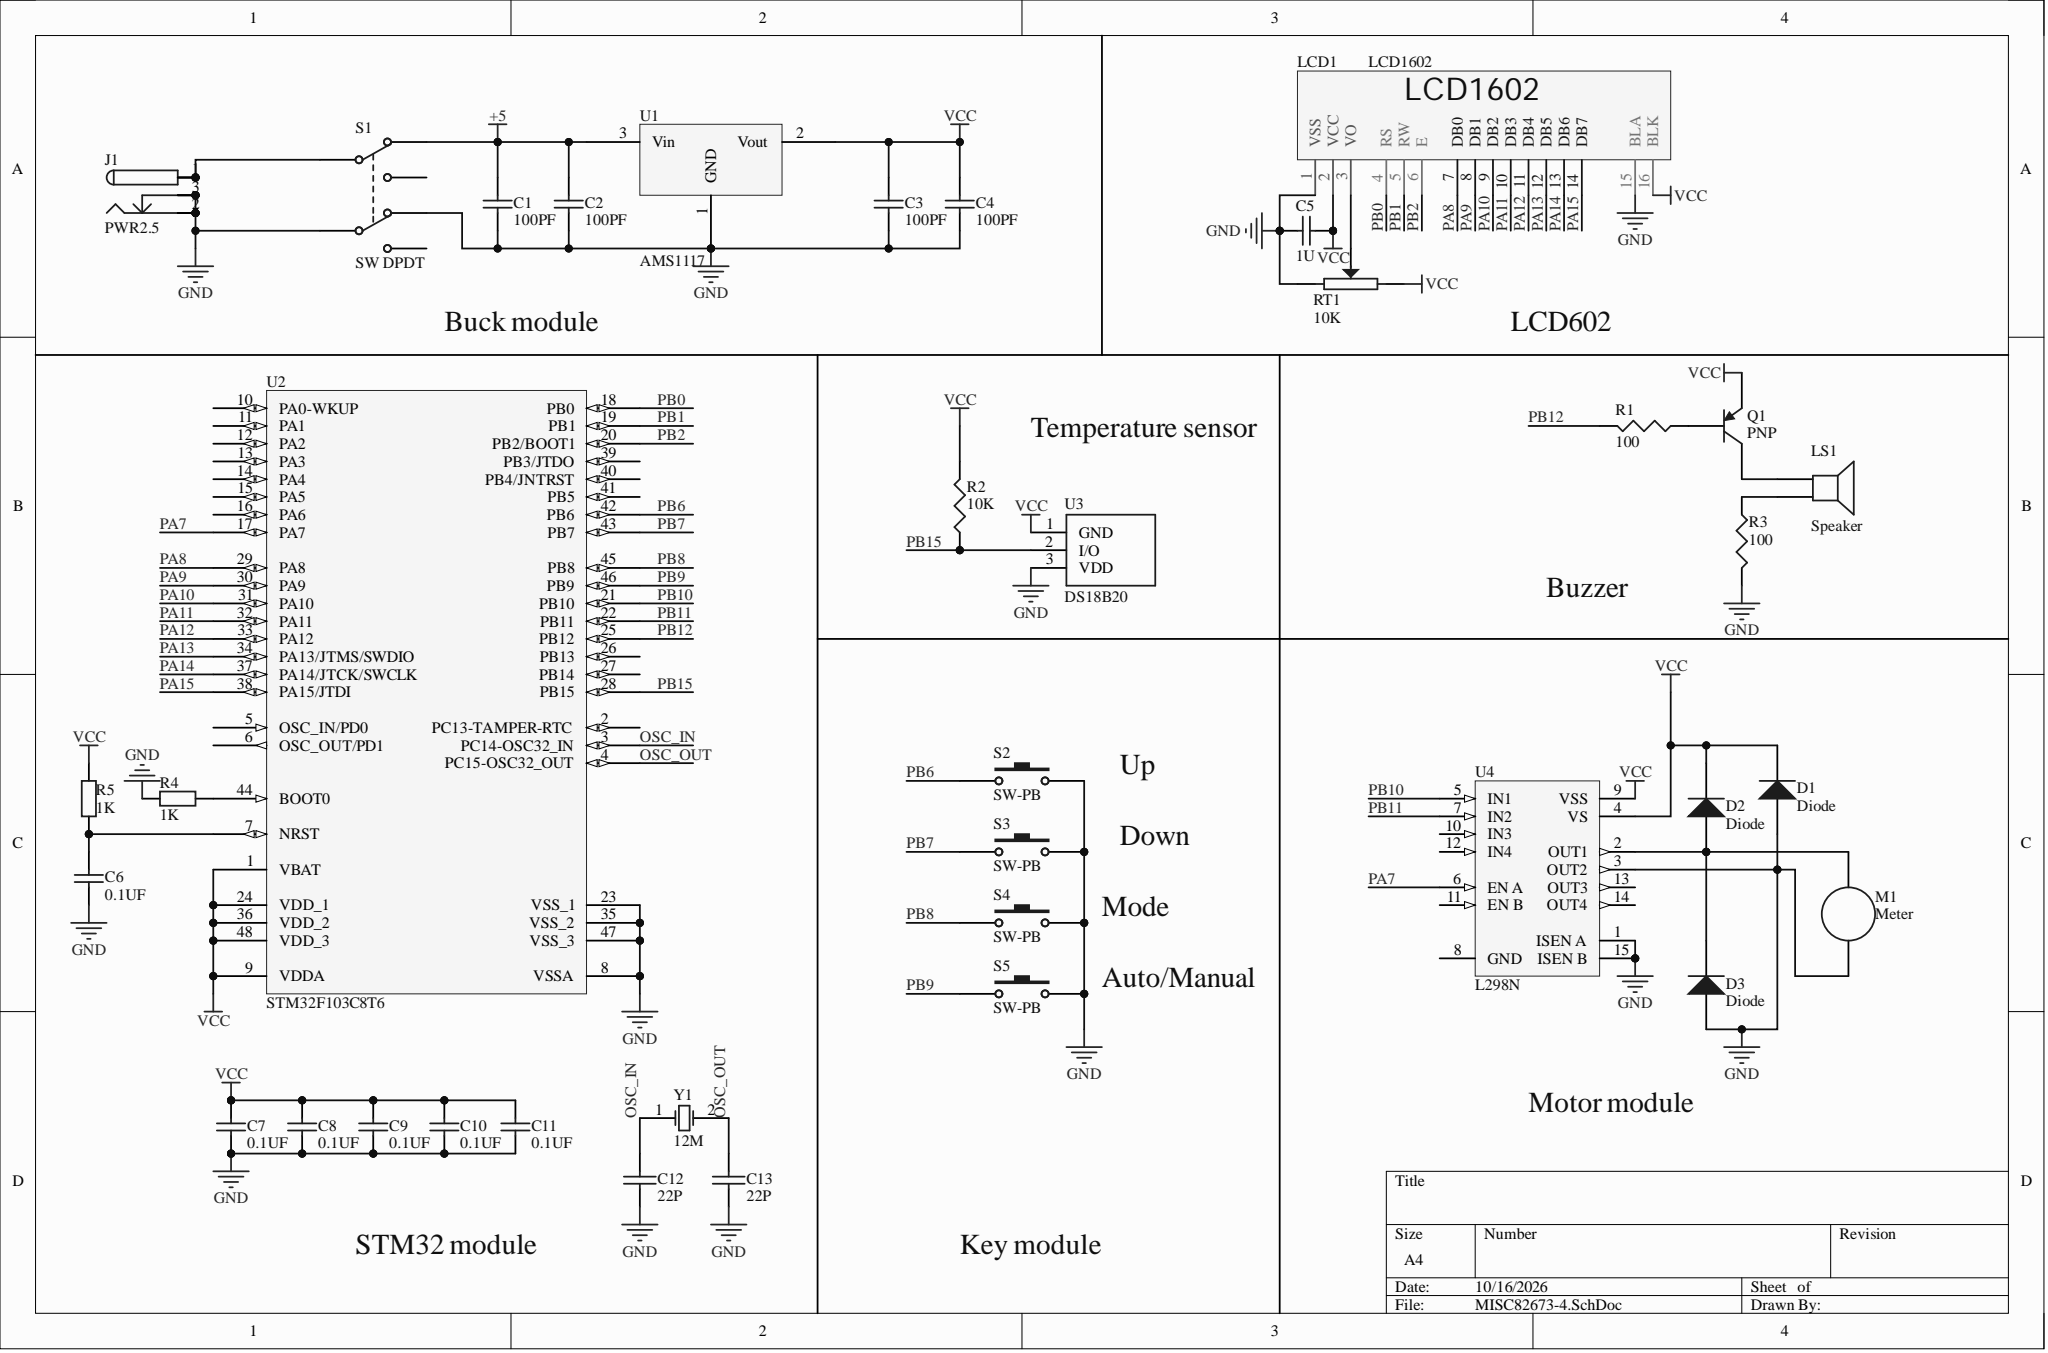Circuit board | Altium Designer | 37 parts | 33 nets
Bill of materials:
Comment,Description,Designator,Footprint,LibRef,Quantity
"100PF","Capacitor (Semiconductor SIM Model)","C1, C2, C3, C4","C1206","Cap Semi","4"
"1U","Capacitor (Semiconductor SIM Model)","C5","C1206","Cap Semi","1"
"0.1UF","Capacitor (Semiconductor SIM Model)","C6, C7, C8, C9, C10, C11","C1206","Cap Semi","6"
"22P","Capacitor","C12, C13","my0603","CAP","2"
"Diode","Default Diode","D1, D2, D3","SMC","Diode","3"
"PWR2.5","Low Voltage Power Supply Connector","J1","KLD-0202","PWR2.5","1"
"LCD1602","","LCD1","LCD1602","LCD1602","1"
"Speaker","Loudspeaker","LS1","PIN2","Speaker","1"
"Meter","Indicating Instrument","M1","RAD-0.1","Meter","1"
"PNP","PNP Bipolar Transistor","Q1","SOT-23B_N","PNP","1"
"100","Resistor","R1, R3","J1-0603","Res3","2"
"10K","Resistor","R2","J1-0603","Res3","1"
"Res2","Resistor","R4, R5","my0603","Res2","2"
"10K","","RT1","电位器","电位器","1"
"SW DPDT","Switch","S1","SOT23-6_N","SW DPDT","1"
"SW-PB","Switch","S2, S3, S4, S5","SW_PB2_A1","SW-PB","4"
"AMS1117","Three-terminal voltage regulator","U1","SOT223","AMS1117","1"
"STM32F103C8T6","","U2","LQFP48 7X7","STM32F103C8T6","1"
"DS18B20","","U3","HDR1X3","DS18B20","1"
"L298N","Dual Full Bridge Driver","U4","Multiwatt15H","L298N","1"
"12M","Crystal Oscillator","Y1","XTAL_US","XTAL","1"
Netlist (Protel format):
[
C1
C1206
100PF



]
[
C2
C1206
100PF



]
[
C3
C1206
100PF



]
[
C4
C1206
100PF



]
[
C5
C1206
1U



]
[
C6
C1206
0.1UF



]
[
C7
C1206
0.1UF



]
[
C8
C1206
0.1UF



]
[
C9
C1206
0.1UF



]
[
C10
C1206
0.1UF



]
[
C11
C1206
0.1UF



]
[
C12
my0603
22P



]
[
C13
my0603
22P



]
[
D1
SMC
Diode



]
[
D2
SMC
Diode



]
[
D3
SMC
Diode



]
[
J1
KLD-0202
PWR2.5



]
[
LCD1
LCD1602
LCD1602



]
[
LS1
PIN2
Speaker



]
[
M1
RAD-0.1
Meter



]
[
Q1
SOT-23B_N
PNP



]
[
R1
J1-0603
100



]
[
R2
J1-0603
10K



]
[
R3
J1-0603
100



]
[
R4
my0603
Res2



]
[
R5
my0603
Res2



]
[
RT1
电位器
10K



]
[
S1
SOT23-6_N
SW DPDT



]
[
S2
SW_PB2_A1
SW-PB



]
[
S3
SW_PB2_A1
SW-PB



]
[
S4
SW_PB2_A1
SW-PB



]
[
S5
SW_PB2_A1
SW-PB



]
[
U1
SOT223
AMS1117



]
[
U2
LQFP48 7X7
STM32F103C8T6



]
[
U3
HDR1X3
DS18B20



]
[
U4
Multiwatt15H
L298N



]
[
Y1
XTAL_US
12M



]
(
VCC
C3-2
C4-2
C5-1
C7-2
C8-2
C9-2
C10-2
C11-2
D1-2
D2-2
LCD1-2
LCD1-16
Q1-3
R2-2
R5-2
RT1-2
U1-2
U2-1
U2-9
U2-24
U2-36
U2-48
U3-1
U4-4
U4-9
)
(
PB15
R2-1
U2-28
U3-2
)
(
PB12
R1-2
U2-25
)
(
PB11
U2-22
U4-7
)
(
PB10
U2-21
U4-5
)
(
PB9
S5-1
U2-46
)
(
PB8
S4-1
U2-45
)
(
PB7
S3-1
U2-43
)
(
PB6
S2-1
U2-42
)
(
PB2
LCD1-6
U2-20
)
(
PB1
LCD1-5
U2-19
)
(
PB0
LCD1-4
U2-18
)
(
PA15
LCD1-14
U2-38
)
(
PA14
LCD1-13
U2-37
)
(
PA13
LCD1-12
U2-34
)
(
PA12
LCD1-11
U2-33
)
(
PA11
LCD1-10
U2-32
)
(
PA10
LCD1-9
U2-31
)
(
PA9
LCD1-8
U2-30
)
(
PA8
LCD1-7
U2-29
)
(
PA7
U2-17
U4-6
)
(
OSC_OUT
C13-1
U2-4
Y1-2
)
(
OSC_IN
C12-1
U2-3
Y1-1
)
(
NetR4_1
R4-1
U2-44
)
(
NetQ1_2
Q1-2
R1-1
)
(
NetLS1_2
LS1-2
R3-1
)
(
NetLS1_1
LS1-1
Q1-1
)
(
NetLCD1_3
LCD1-3
RT1-3
)
(
NetJ1_1
J1-1
J1-1A
J1-1B
S1-1
)
(
NetD2_1
D2-1
D3-2
M1-2
U4-2
)
(
NetC6_2
C6-2
R5-1
U2-7
)
(
GND
C1-1
C2-1
C3-1
C4-1
C5-2
C6-1
C7-1
C8-1
C9-1
C10-1
C11-1
C12-2
C13-2
D1-1
D3-1
J1-2
J1-2A
J1-2B
J1-3
J1-3A
J1-3B
LCD1-1
LCD1-15
M1-1
R3-2
R4-2
RT1-1
S1-4
S1-5
S2-2
S3-2
S4-2
S5-2
U1-1
U2-8
U2-23
U2-35
U2-47
U3-3
U4-1
U4-3
U4-15
)
(
+5
C1-2
C2-2
S1-2
U1-3
)